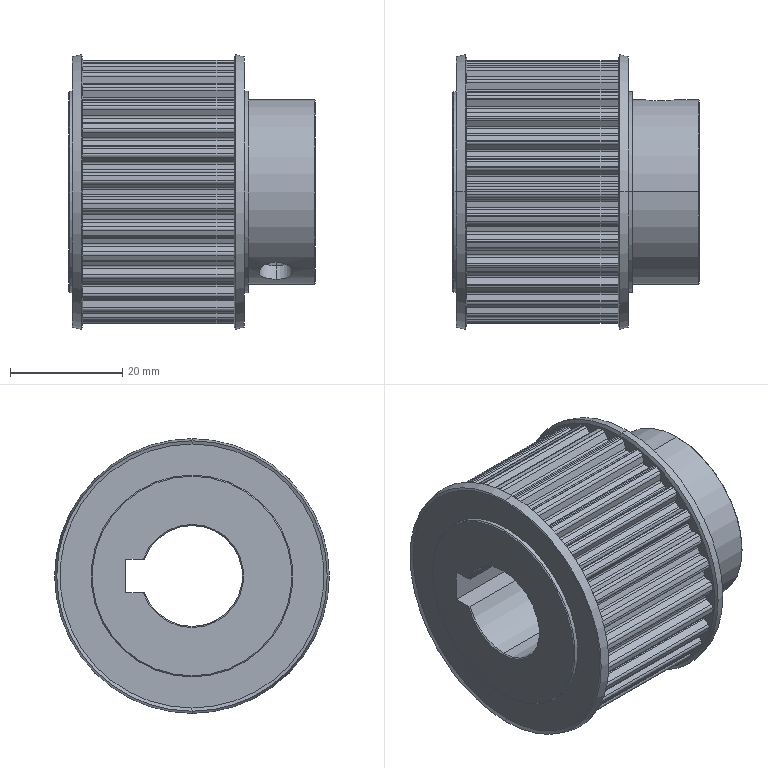Part | STEP file | PN_0012 T5 synchronous pulley 30 teeth 1 | 1 solid | 322 faces | box 44 x 49 x 49 mm | volume 49129 mm3 | cylinder 221 | plane 71 | cone 30 | commonest cylinder face diameters 0.8 x70 1.2 x70 46.95 x31 43.35 x30 6 x7 4.917 x4